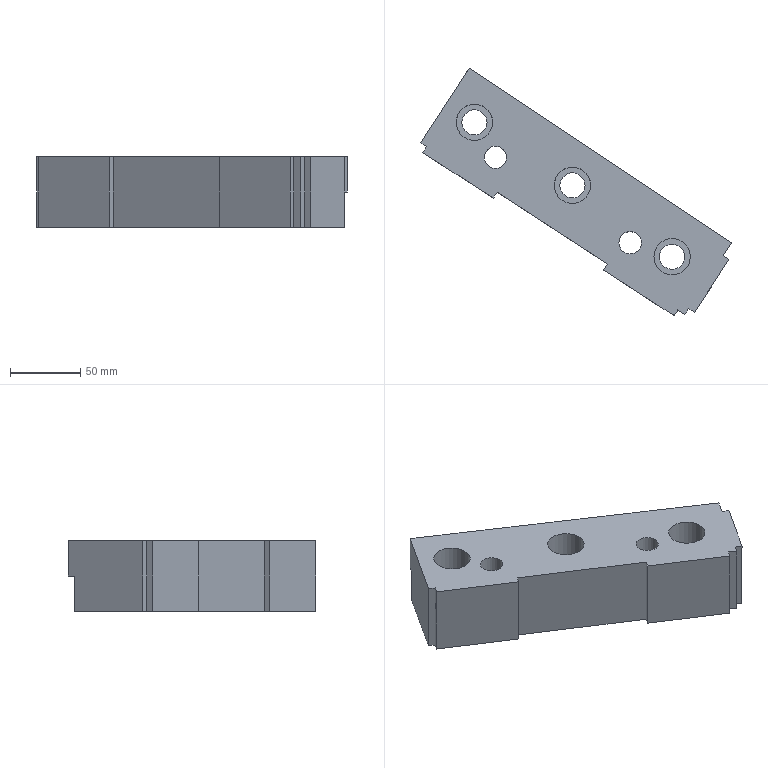Part | NX | features solid 2 | 1 solid | 31 faces | box 221.806 x 176.719 x 50 mm | volume 629014 mm3 | plane 22 | cylinder 8 | spline 1 | commonest cylinder face diameters 18 x3 26 x3 16 x2
STEP:
#1=CARTESIAN_POINT('',(359.804,560.007,-50.));
#2=VERTEX_POINT('',#1);
#3=CARTESIAN_POINT('',(350.804,560.007,-50.));
#4=DIRECTION('',(0.,0.,1.));
#5=DIRECTION('',(1.,0.,0.));
#6=AXIS2_PLACEMENT_3D('',#3,#4,#5);
#7=CIRCLE('',#6,9.);
#8=EDGE_CURVE('',#2,#2,#7,.T.);
#9=ORIENTED_EDGE('',*,*,#8,.F.);
#10=EDGE_LOOP('',(#9));
#11=FACE_BOUND('',#10,.T.);
#12=CARTESIAN_POINT('',(359.804,560.007,-30.));
#13=VERTEX_POINT('',#12);
#14=CARTESIAN_POINT('',(350.804,560.007,-30.));
#15=DIRECTION('',(0.,0.,1.));
#16=DIRECTION('',(1.,0.,0.));
#17=AXIS2_PLACEMENT_3D('',#14,#15,#16);
#18=CIRCLE('',#17,9.);
#19=EDGE_CURVE('',#13,#13,#18,.F.);
#20=ORIENTED_EDGE('',*,*,#19,.F.);
#21=EDGE_LOOP('',(#20));
#22=FACE_BOUND('',#21,.T.);
#23=CARTESIAN_POINT('',(350.804,560.007,-125.));
#24=DIRECTION('',(0.,0.,1.));
#25=DIRECTION('',(1.,0.,0.));
#26=AXIS2_PLACEMENT_3D('',#23,#24,#25);
#27=CYLINDRICAL_SURFACE('',#26,9.);
#28=ADVANCED_FACE('',(#11,#22),#27,.F.);
#29=CARTESIAN_POINT('',(429.804,515.007,-50.));
#30=VERTEX_POINT('',#29);
#31=CARTESIAN_POINT('',(420.804,515.007,-50.));
#32=DIRECTION('',(0.,0.,1.));
#33=DIRECTION('',(1.,0.,0.));
#34=AXIS2_PLACEMENT_3D('',#31,#32,#33);
#35=CIRCLE('',#34,9.);
#36=EDGE_CURVE('',#30,#30,#35,.T.);
#37=ORIENTED_EDGE('',*,*,#36,.F.);
#38=EDGE_LOOP('',(#37));
#39=FACE_BOUND('',#38,.T.);
#40=CARTESIAN_POINT('',(429.804,515.007,-30.));
#41=VERTEX_POINT('',#40);
#42=CARTESIAN_POINT('',(420.804,515.007,-30.));
#43=DIRECTION('',(0.,0.,1.));
#44=DIRECTION('',(1.,0.,0.));
#45=AXIS2_PLACEMENT_3D('',#42,#43,#44);
#46=CIRCLE('',#45,9.);
#47=EDGE_CURVE('',#41,#41,#46,.F.);
#48=ORIENTED_EDGE('',*,*,#47,.F.);
#49=EDGE_LOOP('',(#48));
#50=FACE_BOUND('',#49,.T.);
#51=CARTESIAN_POINT('',(420.804,515.007,-125.));
#52=DIRECTION('',(0.,0.,1.));
#53=DIRECTION('',(1.,0.,0.));
#54=AXIS2_PLACEMENT_3D('',#51,#52,#53);
#55=CYLINDRICAL_SURFACE('',#54,9.);
#56=ADVANCED_FACE('',(#39,#50),#55,.F.);
#57=CARTESIAN_POINT('',(501.017,464.018,-50.));
#58=VERTEX_POINT('',#57);
#59=CARTESIAN_POINT('',(492.017,464.018,-50.));
#60=DIRECTION('',(0.,0.,1.));
#61=DIRECTION('',(1.,0.,0.));
#62=AXIS2_PLACEMENT_3D('',#59,#60,#61);
#63=CIRCLE('',#62,9.);
#64=EDGE_CURVE('',#58,#58,#63,.T.);
#65=ORIENTED_EDGE('',*,*,#64,.F.);
#66=EDGE_LOOP('',(#65));
#67=FACE_BOUND('',#66,.T.);
#68=CARTESIAN_POINT('',(501.017,464.018,-30.));
#69=VERTEX_POINT('',#68);
#70=CARTESIAN_POINT('',(492.017,464.018,-30.));
#71=DIRECTION('',(0.,0.,1.));
#72=DIRECTION('',(1.,0.,0.));
#73=AXIS2_PLACEMENT_3D('',#70,#71,#72);
#74=CIRCLE('',#73,9.);
#75=EDGE_CURVE('',#69,#69,#74,.F.);
#76=ORIENTED_EDGE('',*,*,#75,.F.);
#77=EDGE_LOOP('',(#76));
#78=FACE_BOUND('',#77,.T.);
#79=CARTESIAN_POINT('',(492.017,464.018,-125.));
#80=DIRECTION('',(0.,0.,1.));
#81=DIRECTION('',(1.,0.,0.));
#82=AXIS2_PLACEMENT_3D('',#79,#80,#81);
#83=CYLINDRICAL_SURFACE('',#82,9.);
#84=ADVANCED_FACE('',(#67,#78),#83,.F.);
#85=CARTESIAN_POINT('',(503.876,427.045,-50.));
#86=VERTEX_POINT('',#85);
#87=CARTESIAN_POINT('',(503.876,427.045,0.));
#88=VERTEX_POINT('',#87);
#89=CARTESIAN_POINT('',(503.876,427.045,-50.));
#90=DIRECTION('',(0.,0.,1.));
#91=VECTOR('',#90,1000.);
#92=LINE('',#89,#91);
#93=EDGE_CURVE('',#86,#88,#92,.T.);
#94=ORIENTED_EDGE('',*,*,#93,.T.);
#95=CARTESIAN_POINT('',(501.152,422.852,0.));
#96=VERTEX_POINT('',#95);
#97=CARTESIAN_POINT('',(513.949,442.557,0.));
#98=DIRECTION('',(0.5446,0.8387,0.));
#99=VECTOR('',#98,1000.);
#100=LINE('',#97,#99);
#101=EDGE_CURVE('',#96,#88,#100,.T.);
#102=ORIENTED_EDGE('',*,*,#101,.F.);
#103=CARTESIAN_POINT('',(501.152,422.852,-50.));
#104=VERTEX_POINT('',#103);
#105=CARTESIAN_POINT('',(501.152,422.852,-70.));
#106=DIRECTION('',(0.,0.,1.));
#107=VECTOR('',#106,1000.);
#108=LINE('',#105,#107);
#109=EDGE_CURVE('',#104,#96,#108,.T.);
#110=ORIENTED_EDGE('',*,*,#109,.F.);
#111=CARTESIAN_POINT('',(874.688,998.046,-50.));
#112=DIRECTION('',(-0.5446,-0.8387,0.));
#113=VECTOR('',#112,1000.);
#114=LINE('',#111,#113);
#115=EDGE_CURVE('',#86,#104,#114,.T.);
#116=ORIENTED_EDGE('',*,*,#115,.F.);
#117=EDGE_LOOP('',(#94,#102,#110,#116));
#118=FACE_BOUND('',#117,.T.);
#119=CARTESIAN_POINT('',(1248.625,1573.86,-70.));
#120=DIRECTION('',(-0.8387,0.5446,0.));
#121=DIRECTION('',(-0.5446,-0.8387,0.));
#122=AXIS2_PLACEMENT_3D('',#119,#120,#121);
#123=PLANE('',#122);
#124=ADVANCED_FACE('',(#118),#123,.F.);
#125=CARTESIAN_POINT('',(366.965,509.994,-50.));
#126=VERTEX_POINT('',#125);
#127=CARTESIAN_POINT('',(445.8,458.798,-50.));
#128=VERTEX_POINT('',#127);
#129=CARTESIAN_POINT('',(-52.93,782.677,-50.));
#130=DIRECTION('',(0.8387,-0.5446,0.));
#131=VECTOR('',#130,1000.);
#132=LINE('',#129,#131);
#133=EDGE_CURVE('',#126,#128,#132,.T.);
#134=ORIENTED_EDGE('',*,*,#133,.T.);
#135=CARTESIAN_POINT('',(445.8,458.798,0.));
#136=VERTEX_POINT('',#135);
#137=CARTESIAN_POINT('',(445.8,458.798,-70.));
#138=DIRECTION('',(0.,0.,1.));
#139=VECTOR('',#138,1000.);
#140=LINE('',#137,#139);
#141=EDGE_CURVE('',#128,#136,#140,.T.);
#142=ORIENTED_EDGE('',*,*,#141,.T.);
#143=CARTESIAN_POINT('',(366.965,509.994,0.));
#144=VERTEX_POINT('',#143);
#145=CARTESIAN_POINT('',(-52.93,782.677,0.));
#146=DIRECTION('',(0.8387,-0.5446,0.));
#147=VECTOR('',#146,1000.);
#148=LINE('',#145,#147);
#149=EDGE_CURVE('',#144,#136,#148,.T.);
#150=ORIENTED_EDGE('',*,*,#149,.F.);
#151=CARTESIAN_POINT('',(366.965,509.994,-70.));
#152=DIRECTION('',(0.,0.,1.));
#153=VECTOR('',#152,1000.);
#154=LINE('',#151,#153);
#155=EDGE_CURVE('',#126,#144,#154,.T.);
#156=ORIENTED_EDGE('',*,*,#155,.F.);
#157=EDGE_LOOP('',(#134,#142,#150,#156));
#158=FACE_BOUND('',#157,.T.);
#159=CARTESIAN_POINT('',(-1335.727,1615.736,-70.));
#160=DIRECTION('',(-0.5446,-0.8387,0.));
#161=DIRECTION('',(0.8387,-0.5446,0.));
#162=AXIS2_PLACEMENT_3D('',#159,#160,#161);
#163=PLANE('',#162);
#164=ADVANCED_FACE('',(#158),#163,.T.);
#165=CARTESIAN_POINT('',(312.451,545.396,-50.));
#166=VERTEX_POINT('',#165);
#167=CARTESIAN_POINT('',(316.645,542.673,-50.));
#168=VERTEX_POINT('',#167);
#169=CARTESIAN_POINT('',(-52.93,782.677,-50.));
#170=DIRECTION('',(0.8387,-0.5446,0.));
#171=VECTOR('',#170,1000.);
#172=LINE('',#169,#171);
#173=EDGE_CURVE('',#166,#168,#172,.T.);
#174=ORIENTED_EDGE('',*,*,#173,.T.);
#175=CARTESIAN_POINT('',(316.645,542.673,0.));
#176=VERTEX_POINT('',#175);
#177=CARTESIAN_POINT('',(316.645,542.673,-70.));
#178=DIRECTION('',(0.,0.,1.));
#179=VECTOR('',#178,1000.);
#180=LINE('',#177,#179);
#181=EDGE_CURVE('',#168,#176,#180,.T.);
#182=ORIENTED_EDGE('',*,*,#181,.T.);
#183=CARTESIAN_POINT('',(312.451,545.396,0.));
#184=VERTEX_POINT('',#183);
#185=CARTESIAN_POINT('',(-52.93,782.677,0.));
#186=DIRECTION('',(0.8387,-0.5446,0.));
#187=VECTOR('',#186,1000.);
#188=LINE('',#185,#187);
#189=EDGE_CURVE('',#184,#176,#188,.T.);
#190=ORIENTED_EDGE('',*,*,#189,.F.);
#191=CARTESIAN_POINT('',(312.451,545.396,-70.));
#192=DIRECTION('',(0.,0.,1.));
#193=VECTOR('',#192,1000.);
#194=LINE('',#191,#193);
#195=EDGE_CURVE('',#166,#184,#194,.T.);
#196=ORIENTED_EDGE('',*,*,#195,.F.);
#197=EDGE_LOOP('',(#174,#182,#190,#196));
#198=FACE_BOUND('',#197,.T.);
#199=CARTESIAN_POINT('',(-1335.727,1615.736,-70.));
#200=DIRECTION('',(-0.5446,-0.8387,0.));
#201=DIRECTION('',(0.8387,-0.5446,0.));
#202=AXIS2_PLACEMENT_3D('',#199,#200,#201);
#203=PLANE('',#202);
#204=ADVANCED_FACE('',(#198),#203,.T.);
#205=CARTESIAN_POINT('',(496.12,426.12,-50.));
#206=VERTEX_POINT('',#205);
#207=CARTESIAN_POINT('',(496.12,426.12,0.));
#208=VERTEX_POINT('',#207);
#209=CARTESIAN_POINT('',(496.12,426.12,-70.));
#210=DIRECTION('',(0.,0.,1.));
#211=VECTOR('',#210,1000.);
#212=LINE('',#209,#211);
#213=EDGE_CURVE('',#206,#208,#212,.T.);
#214=ORIENTED_EDGE('',*,*,#213,.F.);
#215=CARTESIAN_POINT('',(-52.93,782.677,-50.));
#216=DIRECTION('',(0.8387,-0.5446,0.));
#217=VECTOR('',#216,1000.);
#218=LINE('',#215,#217);
#219=EDGE_CURVE('',#206,#104,#218,.T.);
#220=ORIENTED_EDGE('',*,*,#219,.T.);
#221=ORIENTED_EDGE('',*,*,#109,.T.);
#222=CARTESIAN_POINT('',(-52.93,782.677,0.));
#223=DIRECTION('',(0.8387,-0.5446,0.));
#224=VECTOR('',#223,1000.);
#225=LINE('',#222,#224);
#226=EDGE_CURVE('',#208,#96,#225,.T.);
#227=ORIENTED_EDGE('',*,*,#226,.F.);
#228=EDGE_LOOP('',(#214,#220,#221,#227));
#229=FACE_BOUND('',#228,.T.);
#230=CARTESIAN_POINT('',(-1335.727,1615.736,-70.));
#231=DIRECTION('',(-0.5446,-0.8387,0.));
#232=DIRECTION('',(0.8387,-0.5446,0.));
#233=AXIS2_PLACEMENT_3D('',#230,#231,#232);
#234=PLANE('',#233);
#235=ADVANCED_FACE('',(#229),#234,.T.);
#236=ORIENTED_EDGE('',*,*,#195,.T.);
#237=CARTESIAN_POINT('',(347.032,598.645,0.));
#238=VERTEX_POINT('',#237);
#239=CARTESIAN_POINT('',(685.987,1120.59,0.));
#240=DIRECTION('',(-0.5446,-0.8387,0.));
#241=VECTOR('',#240,1000.);
#242=LINE('',#239,#241);
#243=EDGE_CURVE('',#238,#184,#242,.T.);
#244=ORIENTED_EDGE('',*,*,#243,.F.);
#245=CARTESIAN_POINT('',(347.032,598.645,-25.));
#246=VERTEX_POINT('',#245);
#247=CARTESIAN_POINT('',(347.032,598.645,-70.));
#248=DIRECTION('',(0.,0.,1.));
#249=VECTOR('',#248,1000.);
#250=LINE('',#247,#249);
#251=EDGE_CURVE('',#246,#238,#250,.T.);
#252=ORIENTED_EDGE('',*,*,#251,.F.);
#253=CARTESIAN_POINT('',(344.309,594.452,-25.));
#254=VERTEX_POINT('',#253);
#255=CARTESIAN_POINT('',(1059.925,1696.404,-25.));
#256=DIRECTION('',(-0.5446,-0.8387,0.));
#257=VECTOR('',#256,1000.);
#258=LINE('',#255,#257);
#259=EDGE_CURVE('',#246,#254,#258,.T.);
#260=ORIENTED_EDGE('',*,*,#259,.T.);
#261=CARTESIAN_POINT('',(344.309,594.452,-50.));
#262=VERTEX_POINT('',#261);
#263=CARTESIAN_POINT('',(344.309,594.452,-70.));
#264=DIRECTION('',(0.,0.,-1.));
#265=VECTOR('',#264,1000.);
#266=LINE('',#263,#265);
#267=EDGE_CURVE('',#254,#262,#266,.T.);
#268=ORIENTED_EDGE('',*,*,#267,.T.);
#269=CARTESIAN_POINT('',(685.987,1120.59,-50.));
#270=DIRECTION('',(-0.5446,-0.8387,0.));
#271=VECTOR('',#270,1000.);
#272=LINE('',#269,#271);
#273=EDGE_CURVE('',#262,#166,#272,.T.);
#274=ORIENTED_EDGE('',*,*,#273,.T.);
#275=EDGE_LOOP('',(#236,#244,#252,#260,#268,#274));
#276=FACE_BOUND('',#275,.T.);
#277=CARTESIAN_POINT('',(1059.925,1696.404,-70.));
#278=DIRECTION('',(-0.8387,0.5446,0.));
#279=DIRECTION('',(-0.5446,-0.8387,0.));
#280=AXIS2_PLACEMENT_3D('',#277,#278,#279);
#281=PLANE('',#280);
#282=ADVANCED_FACE('',(#276),#281,.T.);
#283=CARTESIAN_POINT('',(534.257,473.829,-25.));
#284=VERTEX_POINT('',#283);
#285=CARTESIAN_POINT('',(347.032,598.645,-25.));
#286=DIRECTION('',(0.8321,-0.5547,0.));
#287=VECTOR('',#286,1000.);
#288=LINE('',#285,#287);
#289=EDGE_CURVE('',#246,#284,#288,.T.);
#290=ORIENTED_EDGE('',*,*,#289,.F.);
#291=ORIENTED_EDGE('',*,*,#251,.T.);
#292=CARTESIAN_POINT('',(534.257,473.829,0.));
#293=VERTEX_POINT('',#292);
#294=CARTESIAN_POINT('',(-21.675,844.45,0.));
#295=DIRECTION('',(0.8321,-0.5547,0.));
#296=VECTOR('',#295,1000.);
#297=LINE('',#294,#296);
#298=EDGE_CURVE('',#238,#293,#297,.T.);
#299=ORIENTED_EDGE('',*,*,#298,.T.);
#300=CARTESIAN_POINT('',(534.257,473.829,-70.));
#301=DIRECTION('',(0.,0.,1.));
#302=VECTOR('',#301,1000.);
#303=LINE('',#300,#302);
#304=EDGE_CURVE('',#284,#293,#303,.T.);
#305=ORIENTED_EDGE('',*,*,#304,.F.);
#306=EDGE_LOOP('',(#290,#291,#299,#305));
#307=FACE_BOUND('',#306,.T.);
#308=CARTESIAN_POINT('',(347.032,598.645,-70.));
#309=DIRECTION('',(-0.5547,-0.8321,0.));
#310=DIRECTION('',(0.8321,-0.5547,0.));
#311=AXIS2_PLACEMENT_3D('',#308,#309,#310);
#312=PLANE('',#311);
#313=ADVANCED_FACE('',(#307),#312,.F.);
#314=ORIENTED_EDGE('',*,*,#8,.T.);
#315=EDGE_LOOP('',(#314));
#316=FACE_BOUND('',#315,.T.);
#317=CARTESIAN_POINT('',(373.804,535.007,-50.));
#318=VERTEX_POINT('',#317);
#319=CARTESIAN_POINT('',(365.804,535.007,-50.));
#320=DIRECTION('',(0.,0.,1.));
#321=DIRECTION('',(1.,0.,0.));
#322=AXIS2_PLACEMENT_3D('',#319,#320,#321);
#323=CIRCLE('',#322,8.);
#324=EDGE_CURVE('',#318,#318,#323,.T.);
#325=ORIENTED_EDGE('',*,*,#324,.T.);
#326=EDGE_LOOP('',(#325));
#327=FACE_BOUND('',#326,.T.);
#328=ORIENTED_EDGE('',*,*,#36,.T.);
#329=EDGE_LOOP('',(#328));
#330=FACE_BOUND('',#329,.T.);
#331=CARTESIAN_POINT('',(470.017,474.018,-50.));
#332=VERTEX_POINT('',#331);
#333=CARTESIAN_POINT('',(462.017,474.018,-50.));
#334=DIRECTION('',(0.,0.,1.));
#335=DIRECTION('',(1.,0.,0.));
#336=AXIS2_PLACEMENT_3D('',#333,#334,#335);
#337=CIRCLE('',#336,8.);
#338=EDGE_CURVE('',#332,#332,#337,.T.);
#339=ORIENTED_EDGE('',*,*,#338,.T.);
#340=EDGE_LOOP('',(#339));
#341=FACE_BOUND('',#340,.T.);
#342=ORIENTED_EDGE('',*,*,#64,.T.);
#343=EDGE_LOOP('',(#342));
#344=FACE_BOUND('',#343,.T.);
#345=CARTESIAN_POINT('',(531.534,469.635,-50.));
#346=VERTEX_POINT('',#345);
#347=CARTESIAN_POINT('',(344.309,594.452,-50.));
#348=CARTESIAN_POINT('',(406.717,552.846,-50.));
#349=CARTESIAN_POINT('',(469.125,511.241,-50.));
#350=CARTESIAN_POINT('',(531.534,469.635,-50.));
#351=B_SPLINE_CURVE_WITH_KNOTS('',3,(#347,#348,#349,#350),.UNSPECIFIED.,.F.,.F.,(4,4),(0.,1.),.UNSPECIFIED.);
#352=EDGE_CURVE('',#262,#346,#351,.T.);
#353=ORIENTED_EDGE('',*,*,#352,.T.);
#354=CARTESIAN_POINT('',(528.384,464.786,-50.));
#355=VERTEX_POINT('',#354);
#356=CARTESIAN_POINT('',(874.688,998.046,-50.));
#357=DIRECTION('',(-0.5446,-0.8387,0.));
#358=VECTOR('',#357,1000.);
#359=LINE('',#356,#358);
#360=EDGE_CURVE('',#346,#355,#359,.T.);
#361=ORIENTED_EDGE('',*,*,#360,.T.);
#362=CARTESIAN_POINT('',(532.578,462.062,-50.));
#363=VERTEX_POINT('',#362);
#364=CARTESIAN_POINT('',(528.384,464.786,-50.));
#365=DIRECTION('',(0.8387,-0.5446,0.));
#366=VECTOR('',#365,1000.);
#367=LINE('',#364,#366);
#368=EDGE_CURVE('',#355,#363,#367,.T.);
#369=ORIENTED_EDGE('',*,*,#368,.T.);
#370=CARTESIAN_POINT('',(508.069,424.322,-50.));
#371=VERTEX_POINT('',#370);
#372=CARTESIAN_POINT('',(503.712,417.613,-50.));
#373=DIRECTION('',(0.5446,0.8387,0.));
#374=VECTOR('',#373,1000.);
#375=LINE('',#372,#374);
#376=EDGE_CURVE('',#371,#363,#375,.T.);
#377=ORIENTED_EDGE('',*,*,#376,.F.);
#378=CARTESIAN_POINT('',(503.876,427.045,-50.));
#379=DIRECTION('',(0.8387,-0.5446,0.));
#380=VECTOR('',#379,1000.);
#381=LINE('',#378,#380);
#382=EDGE_CURVE('',#86,#371,#381,.T.);
#383=ORIENTED_EDGE('',*,*,#382,.F.);
#384=ORIENTED_EDGE('',*,*,#115,.T.);
#385=ORIENTED_EDGE('',*,*,#219,.F.);
#386=CARTESIAN_POINT('',(493.397,421.926,-50.));
#387=VERTEX_POINT('',#386);
#388=CARTESIAN_POINT('',(485.228,409.346,-50.));
#389=DIRECTION('',(-0.5446,-0.8387,0.));
#390=VECTOR('',#389,1000.);
#391=LINE('',#388,#390);
#392=EDGE_CURVE('',#206,#387,#391,.T.);
#393=ORIENTED_EDGE('',*,*,#392,.T.);
#394=CARTESIAN_POINT('',(443.077,454.605,-50.));
#395=VERTEX_POINT('',#394);
#396=CARTESIAN_POINT('',(468.237,438.266,-50.));
#397=DIRECTION('',(0.8387,-0.5446,0.));
#398=VECTOR('',#397,1000.);
#399=LINE('',#396,#398);
#400=EDGE_CURVE('',#395,#387,#399,.T.);
#401=ORIENTED_EDGE('',*,*,#400,.F.);
#402=CARTESIAN_POINT('',(434.907,442.025,-50.));
#403=DIRECTION('',(-0.5446,-0.8387,0.));
#404=VECTOR('',#403,1000.);
#405=LINE('',#402,#404);
#406=EDGE_CURVE('',#128,#395,#405,.T.);
#407=ORIENTED_EDGE('',*,*,#406,.F.);
#408=ORIENTED_EDGE('',*,*,#133,.F.);
#409=CARTESIAN_POINT('',(364.242,505.801,-50.));
#410=VERTEX_POINT('',#409);
#411=CARTESIAN_POINT('',(356.072,493.221,-50.));
#412=DIRECTION('',(-0.5446,-0.8387,0.));
#413=VECTOR('',#412,1000.);
#414=LINE('',#411,#413);
#415=EDGE_CURVE('',#126,#410,#414,.T.);
#416=ORIENTED_EDGE('',*,*,#415,.T.);
#417=CARTESIAN_POINT('',(313.922,538.479,-50.));
#418=VERTEX_POINT('',#417);
#419=CARTESIAN_POINT('',(322.308,533.033,-50.));
#420=DIRECTION('',(0.8387,-0.5446,0.));
#421=VECTOR('',#420,1000.);
#422=LINE('',#419,#421);
#423=EDGE_CURVE('',#418,#410,#422,.T.);
#424=ORIENTED_EDGE('',*,*,#423,.F.);
#425=CARTESIAN_POINT('',(305.752,525.899,-50.));
#426=DIRECTION('',(-0.5446,-0.8387,0.));
#427=VECTOR('',#426,1000.);
#428=LINE('',#425,#427);
#429=EDGE_CURVE('',#168,#418,#428,.T.);
#430=ORIENTED_EDGE('',*,*,#429,.F.);
#431=ORIENTED_EDGE('',*,*,#173,.F.);
#432=ORIENTED_EDGE('',*,*,#273,.F.);
#433=EDGE_LOOP('',(#353,#361,#369,#377,#383,#384,#385,#393,#401,#407,#408,#416,#424,#430,#431,#432));
#434=FACE_BOUND('',#433,.T.);
#435=CARTESIAN_POINT('',(320.605,1357.871,-50.));
#436=DIRECTION('',(0.,0.,1.));
#437=DIRECTION('',(1.,0.,0.));
#438=AXIS2_PLACEMENT_3D('',#435,#436,#437);
#439=PLANE('',#438);
#440=ADVANCED_FACE('',(#316,#327,#330,#341,#344,#434),#439,.F.);
#441=CARTESIAN_POINT('',(528.384,464.786,0.));
#442=VERTEX_POINT('',#441);
#443=CARTESIAN_POINT('',(874.688,998.046,0.));
#444=DIRECTION('',(-0.5446,-0.8387,0.));
#445=VECTOR('',#444,1000.);
#446=LINE('',#443,#445);
#447=EDGE_CURVE('',#293,#442,#446,.T.);
#448=ORIENTED_EDGE('',*,*,#447,.T.);
#449=CARTESIAN_POINT('',(528.384,464.786,-50.));
#450=DIRECTION('',(0.,0.,1.));
#451=VECTOR('',#450,1000.);
#452=LINE('',#449,#451);
#453=EDGE_CURVE('',#355,#442,#452,.T.);
#454=ORIENTED_EDGE('',*,*,#453,.F.);
#455=ORIENTED_EDGE('',*,*,#360,.F.);
#456=CARTESIAN_POINT('',(531.534,469.635,-25.));
#457=VERTEX_POINT('',#456);
#458=CARTESIAN_POINT('',(531.534,469.635,-37.5));
#459=DIRECTION('',(0.,0.,-1.));
#460=VECTOR('',#459,1000.);
#461=LINE('',#458,#460);
#462=EDGE_CURVE('',#457,#346,#461,.T.);
#463=ORIENTED_EDGE('',*,*,#462,.F.);
#464=CARTESIAN_POINT('',(1248.625,1573.86,-25.));
#465=DIRECTION('',(-0.5446,-0.8387,0.));
#466=VECTOR('',#465,1000.);
#467=LINE('',#464,#466);
#468=EDGE_CURVE('',#284,#457,#467,.T.);
#469=ORIENTED_EDGE('',*,*,#468,.F.);
#470=ORIENTED_EDGE('',*,*,#304,.T.);
#471=EDGE_LOOP('',(#448,#454,#455,#463,#469,#470));
#472=FACE_BOUND('',#471,.T.);
#473=CARTESIAN_POINT('',(1248.625,1573.86,-70.));
#474=DIRECTION('',(-0.8387,0.5446,0.));
#475=DIRECTION('',(-0.5446,-0.8387,0.));
#476=AXIS2_PLACEMENT_3D('',#473,#474,#475);
#477=PLANE('',#476);
#478=ADVANCED_FACE('',(#472),#477,.F.);
#479=ORIENTED_EDGE('',*,*,#243,.T.);
#480=ORIENTED_EDGE('',*,*,#189,.T.);
#481=CARTESIAN_POINT('',(313.922,538.479,0.));
#482=VERTEX_POINT('',#481);
#483=CARTESIAN_POINT('',(329.441,562.378,0.));
#484=DIRECTION('',(-0.5446,-0.8387,0.));
#485=VECTOR('',#484,1000.);
#486=LINE('',#483,#485);
#487=EDGE_CURVE('',#176,#482,#486,.T.);
#488=ORIENTED_EDGE('',*,*,#487,.T.);
#489=CARTESIAN_POINT('',(364.242,505.801,0.));
#490=VERTEX_POINT('',#489);
#491=CARTESIAN_POINT('',(322.308,533.033,0.));
#492=DIRECTION('',(0.8387,-0.5446,0.));
#493=VECTOR('',#492,1000.);
#494=LINE('',#491,#493);
#495=EDGE_CURVE('',#482,#490,#494,.T.);
#496=ORIENTED_EDGE('',*,*,#495,.T.);
#497=CARTESIAN_POINT('',(379.762,529.699,0.));
#498=DIRECTION('',(-0.5446,-0.8387,0.));
#499=VECTOR('',#498,1000.);
#500=LINE('',#497,#499);
#501=EDGE_CURVE('',#144,#490,#500,.T.);
#502=ORIENTED_EDGE('',*,*,#501,.F.);
#503=ORIENTED_EDGE('',*,*,#149,.T.);
#504=CARTESIAN_POINT('',(443.077,454.605,0.));
#505=VERTEX_POINT('',#504);
#506=CARTESIAN_POINT('',(458.597,478.503,0.));
#507=DIRECTION('',(-0.5446,-0.8387,0.));
#508=VECTOR('',#507,1000.);
#509=LINE('',#506,#508);
#510=EDGE_CURVE('',#136,#505,#509,.T.);
#511=ORIENTED_EDGE('',*,*,#510,.T.);
#512=CARTESIAN_POINT('',(493.397,421.926,0.));
#513=VERTEX_POINT('',#512);
#514=CARTESIAN_POINT('',(468.237,438.266,0.));
#515=DIRECTION('',(0.8387,-0.5446,0.));
#516=VECTOR('',#515,1000.);
#517=LINE('',#514,#516);
#518=EDGE_CURVE('',#505,#513,#517,.T.);
#519=ORIENTED_EDGE('',*,*,#518,.T.);
#520=CARTESIAN_POINT('',(508.917,445.825,0.));
#521=DIRECTION('',(-0.5446,-0.8387,0.));
#522=VECTOR('',#521,1000.);
#523=LINE('',#520,#522);
#524=EDGE_CURVE('',#208,#513,#523,.T.);
#525=ORIENTED_EDGE('',*,*,#524,.F.);
#526=ORIENTED_EDGE('',*,*,#226,.T.);
#527=ORIENTED_EDGE('',*,*,#101,.T.);
#528=CARTESIAN_POINT('',(508.069,424.322,0.));
#529=VERTEX_POINT('',#528);
#530=CARTESIAN_POINT('',(503.876,427.045,0.));
#531=DIRECTION('',(0.8387,-0.5446,0.));
#532=VECTOR('',#531,1000.);
#533=LINE('',#530,#532);
#534=EDGE_CURVE('',#88,#529,#533,.T.);
#535=ORIENTED_EDGE('',*,*,#534,.T.);
#536=CARTESIAN_POINT('',(532.578,462.062,0.));
#537=VERTEX_POINT('',#536);
#538=CARTESIAN_POINT('',(518.142,439.834,0.));
#539=DIRECTION('',(0.5446,0.8387,0.));
#540=VECTOR('',#539,1000.);
#541=LINE('',#538,#540);
#542=EDGE_CURVE('',#529,#537,#541,.T.);
#543=ORIENTED_EDGE('',*,*,#542,.T.);
#544=CARTESIAN_POINT('',(528.384,464.786,0.));
#545=DIRECTION('',(0.8387,-0.5446,0.));
#546=VECTOR('',#545,1000.);
#547=LINE('',#544,#546);
#548=EDGE_CURVE('',#442,#537,#547,.T.);
#549=ORIENTED_EDGE('',*,*,#548,.F.);
#550=ORIENTED_EDGE('',*,*,#447,.F.);
#551=ORIENTED_EDGE('',*,*,#298,.F.);
#552=EDGE_LOOP('',(#479,#480,#488,#496,#502,#503,#511,#519,#525,#526,#527,#535,#543,#549,#550,#551));
#553=FACE_BOUND('',#552,.T.);
#554=CARTESIAN_POINT('',(337.804,560.007,0.));
#555=VERTEX_POINT('',#554);
#556=CARTESIAN_POINT('',(350.804,560.007,0.));
#557=DIRECTION('',(0.,0.,-1.));
#558=DIRECTION('',(-1.,0.,0.));
#559=AXIS2_PLACEMENT_3D('',#556,#557,#558);
#560=CIRCLE('',#559,13.);
#561=EDGE_CURVE('',#555,#555,#560,.F.);
#562=ORIENTED_EDGE('',*,*,#561,.F.);
#563=EDGE_LOOP('',(#562));
#564=FACE_BOUND('',#563,.T.);
#565=CARTESIAN_POINT('',(407.804,515.007,0.));
#566=VERTEX_POINT('',#565);
#567=CARTESIAN_POINT('',(420.804,515.007,0.));
#568=DIRECTION('',(0.,0.,-1.));
#569=DIRECTION('',(-1.,0.,0.));
#570=AXIS2_PLACEMENT_3D('',#567,#568,#569);
#571=CIRCLE('',#570,13.);
#572=EDGE_CURVE('',#566,#566,#571,.F.);
#573=ORIENTED_EDGE('',*,*,#572,.F.);
#574=EDGE_LOOP('',(#573));
#575=FACE_BOUND('',#574,.T.);
#576=CARTESIAN_POINT('',(479.017,464.018,0.));
#577=VERTEX_POINT('',#576);
#578=CARTESIAN_POINT('',(492.017,464.018,0.));
#579=DIRECTION('',(0.,0.,-1.));
#580=DIRECTION('',(-1.,0.,0.));
#581=AXIS2_PLACEMENT_3D('',#578,#579,#580);
#582=CIRCLE('',#581,13.);
#583=EDGE_CURVE('',#577,#577,#582,.F.);
#584=ORIENTED_EDGE('',*,*,#583,.F.);
#585=EDGE_LOOP('',(#584));
#586=FACE_BOUND('',#585,.T.);
#587=CARTESIAN_POINT('',(357.804,535.007,0.));
#588=VERTEX_POINT('',#587);
#589=CARTESIAN_POINT('',(365.804,535.007,0.));
#590=DIRECTION('',(0.,0.,-1.));
#591=DIRECTION('',(-1.,0.,0.));
#592=AXIS2_PLACEMENT_3D('',#589,#590,#591);
#593=CIRCLE('',#592,8.);
#594=EDGE_CURVE('',#588,#588,#593,.F.);
#595=ORIENTED_EDGE('',*,*,#594,.F.);
#596=EDGE_LOOP('',(#595));
#597=FACE_BOUND('',#596,.T.);
#598=CARTESIAN_POINT('',(454.017,474.018,0.));
#599=VERTEX_POINT('',#598);
#600=CARTESIAN_POINT('',(462.017,474.018,0.));
#601=DIRECTION('',(0.,0.,-1.));
#602=DIRECTION('',(-1.,0.,0.));
#603=AXIS2_PLACEMENT_3D('',#600,#601,#602);
#604=CIRCLE('',#603,8.);
#605=EDGE_CURVE('',#599,#599,#604,.F.);
#606=ORIENTED_EDGE('',*,*,#605,.F.);
#607=EDGE_LOOP('',(#606));
#608=FACE_BOUND('',#607,.T.);
#609=CARTESIAN_POINT('',(320.605,1357.871,0.));
#610=DIRECTION('',(0.,0.,1.));
#611=DIRECTION('',(1.,0.,0.));
#612=AXIS2_PLACEMENT_3D('',#609,#610,#611);
#613=PLANE('',#612);
#614=ADVANCED_FACE('',(#553,#564,#575,#586,#597,#608),#613,.T.);
#615=CARTESIAN_POINT('',(344.309,594.452,-25.));
#616=CARTESIAN_POINT('',(406.717,552.846,-25.));
#617=CARTESIAN_POINT('',(469.125,511.241,-25.));
#618=CARTESIAN_POINT('',(531.534,469.635,-25.));
#619=B_SPLINE_CURVE_WITH_KNOTS('',3,(#615,#616,#617,#618),.UNSPECIFIED.,.F.,.F.,(4,4),(0.9632,1.188),.UNSPECIFIED.);
#620=EDGE_CURVE('',#254,#457,#619,.T.);
#621=ORIENTED_EDGE('',*,*,#620,.T.);
#622=ORIENTED_EDGE('',*,*,#462,.T.);
#623=ORIENTED_EDGE('',*,*,#352,.F.);
#624=ORIENTED_EDGE('',*,*,#267,.F.);
#625=EDGE_LOOP('',(#621,#622,#623,#624));
#626=FACE_BOUND('',#625,.T.);
#627=CARTESIAN_POINT('',(344.309,594.452,-25.));
#628=CARTESIAN_POINT('',(344.309,594.452,-50.));
#629=CARTESIAN_POINT('',(411.082,549.936,-25.));
#630=CARTESIAN_POINT('',(411.082,549.936,-50.));
#631=CARTESIAN_POINT('',(465.216,513.847,-25.));
#632=CARTESIAN_POINT('',(465.216,513.847,-50.));
#633=CARTESIAN_POINT('',(531.534,469.635,-25.));
#634=CARTESIAN_POINT('',(531.534,469.635,-50.));
#635=B_SPLINE_SURFACE_WITH_KNOTS('',3,1,((#627,#628),(#629,#630),(#631,#632),(#633,#634)),.SURF_OF_LINEAR_EXTRUSION.,.F.,.F.,.F.,(4,4),(2,2),(0.0002501,1.),(0.,1.),.PIECEWISE_BEZIER_KNOTS.);
#636=ADVANCED_FACE('',(#626),#635,.T.);
#637=ORIENTED_EDGE('',*,*,#289,.T.);
#638=ORIENTED_EDGE('',*,*,#468,.T.);
#639=ORIENTED_EDGE('',*,*,#620,.F.);
#640=ORIENTED_EDGE('',*,*,#259,.F.);
#641=EDGE_LOOP('',(#637,#638,#639,#640));
#642=FACE_BOUND('',#641,.T.);
#643=CARTESIAN_POINT('',(347.032,598.645,-25.));
#644=DIRECTION('',(0.,0.,-1.));
#645=DIRECTION('',(-1.,0.,0.));
#646=AXIS2_PLACEMENT_3D('',#643,#644,#645);
#647=PLANE('',#646);
#648=ADVANCED_FACE('',(#642),#647,.T.);
#649=CARTESIAN_POINT('',(364.242,505.801,-50.));
#650=DIRECTION('',(0.,0.,1.));
#651=VECTOR('',#650,1000.);
#652=LINE('',#649,#651);
#653=EDGE_CURVE('',#410,#490,#652,.T.);
#654=ORIENTED_EDGE('',*,*,#653,.F.);
#655=ORIENTED_EDGE('',*,*,#415,.F.);
#656=ORIENTED_EDGE('',*,*,#155,.T.);
#657=ORIENTED_EDGE('',*,*,#501,.T.);
#658=EDGE_LOOP('',(#654,#655,#656,#657));
#659=FACE_BOUND('',#658,.T.);
#660=CARTESIAN_POINT('',(356.072,493.221,-50.));
#661=DIRECTION('',(0.8387,-0.5446,0.));
#662=DIRECTION('',(0.5446,0.8387,0.));
#663=AXIS2_PLACEMENT_3D('',#660,#661,#662);
#664=PLANE('',#663);
#665=ADVANCED_FACE('',(#659),#664,.T.);
#666=CARTESIAN_POINT('',(313.922,538.479,-50.));
#667=DIRECTION('',(0.,0.,1.));
#668=VECTOR('',#667,1000.);
#669=LINE('',#666,#668);
#670=EDGE_CURVE('',#418,#482,#669,.T.);
#671=ORIENTED_EDGE('',*,*,#670,.T.);
#672=ORIENTED_EDGE('',*,*,#487,.F.);
#673=ORIENTED_EDGE('',*,*,#181,.F.);
#674=ORIENTED_EDGE('',*,*,#429,.T.);
#675=EDGE_LOOP('',(#671,#672,#673,#674));
#676=FACE_BOUND('',#675,.T.);
#677=CARTESIAN_POINT('',(305.752,525.899,-50.));
#678=DIRECTION('',(0.8387,-0.5446,0.));
#679=DIRECTION('',(0.5446,0.8387,0.));
#680=AXIS2_PLACEMENT_3D('',#677,#678,#679);
#681=PLANE('',#680);
#682=ADVANCED_FACE('',(#676),#681,.F.);
#683=ORIENTED_EDGE('',*,*,#653,.T.);
#684=ORIENTED_EDGE('',*,*,#495,.F.);
#685=ORIENTED_EDGE('',*,*,#670,.F.);
#686=ORIENTED_EDGE('',*,*,#423,.T.);
#687=EDGE_LOOP('',(#683,#684,#685,#686));
#688=FACE_BOUND('',#687,.T.);
#689=CARTESIAN_POINT('',(322.308,533.033,-50.));
#690=DIRECTION('',(0.5446,0.8387,0.));
#691=DIRECTION('',(0.,0.,1.));
#692=AXIS2_PLACEMENT_3D('',#689,#690,#691);
#693=PLANE('',#692);
#694=ADVANCED_FACE('',(#688),#693,.F.);
#695=CARTESIAN_POINT('',(493.397,421.926,-50.));
#696=DIRECTION('',(0.,0.,1.));
#697=VECTOR('',#696,1000.);
#698=LINE('',#695,#697);
#699=EDGE_CURVE('',#387,#513,#698,.T.);
#700=ORIENTED_EDGE('',*,*,#699,.F.);
#701=ORIENTED_EDGE('',*,*,#392,.F.);
#702=ORIENTED_EDGE('',*,*,#213,.T.);
#703=ORIENTED_EDGE('',*,*,#524,.T.);
#704=EDGE_LOOP('',(#700,#701,#702,#703));
#705=FACE_BOUND('',#704,.T.);
#706=CARTESIAN_POINT('',(485.228,409.346,-50.));
#707=DIRECTION('',(0.8387,-0.5446,0.));
#708=DIRECTION('',(0.5446,0.8387,0.));
#709=AXIS2_PLACEMENT_3D('',#706,#707,#708);
#710=PLANE('',#709);
#711=ADVANCED_FACE('',(#705),#710,.T.);
#712=CARTESIAN_POINT('',(443.077,454.605,-50.));
#713=DIRECTION('',(0.,0.,1.));
#714=VECTOR('',#713,1000.);
#715=LINE('',#712,#714);
#716=EDGE_CURVE('',#395,#505,#715,.T.);
#717=ORIENTED_EDGE('',*,*,#716,.T.);
#718=ORIENTED_EDGE('',*,*,#510,.F.);
#719=ORIENTED_EDGE('',*,*,#141,.F.);
#720=ORIENTED_EDGE('',*,*,#406,.T.);
#721=EDGE_LOOP('',(#717,#718,#719,#720));
#722=FACE_BOUND('',#721,.T.);
#723=CARTESIAN_POINT('',(434.907,442.025,-50.));
#724=DIRECTION('',(0.8387,-0.5446,0.));
#725=DIRECTION('',(0.5446,0.8387,0.));
#726=AXIS2_PLACEMENT_3D('',#723,#724,#725);
#727=PLANE('',#726);
#728=ADVANCED_FACE('',(#722),#727,.F.);
#729=ORIENTED_EDGE('',*,*,#699,.T.);
#730=ORIENTED_EDGE('',*,*,#518,.F.);
#731=ORIENTED_EDGE('',*,*,#716,.F.);
#732=ORIENTED_EDGE('',*,*,#400,.T.);
#733=EDGE_LOOP('',(#729,#730,#731,#732));
#734=FACE_BOUND('',#733,.T.);
#735=CARTESIAN_POINT('',(468.237,438.266,-50.));
#736=DIRECTION('',(0.5446,0.8387,0.));
#737=DIRECTION('',(0.,0.,1.));
#738=AXIS2_PLACEMENT_3D('',#735,#736,#737);
#739=PLANE('',#738);
#740=ADVANCED_FACE('',(#734),#739,.F.);
#741=CARTESIAN_POINT('',(532.578,462.062,-50.));
#742=DIRECTION('',(0.,0.,1.));
#743=VECTOR('',#742,1000.);
#744=LINE('',#741,#743);
#745=EDGE_CURVE('',#363,#537,#744,.T.);
#746=ORIENTED_EDGE('',*,*,#745,.F.);
#747=ORIENTED_EDGE('',*,*,#368,.F.);
#748=ORIENTED_EDGE('',*,*,#453,.T.);
#749=ORIENTED_EDGE('',*,*,#548,.T.);
#750=EDGE_LOOP('',(#746,#747,#748,#749));
#751=FACE_BOUND('',#750,.T.);
#752=CARTESIAN_POINT('',(528.384,464.786,-50.));
#753=DIRECTION('',(0.5446,0.8387,0.));
#754=DIRECTION('',(-0.8387,0.5446,0.));
#755=AXIS2_PLACEMENT_3D('',#752,#753,#754);
#756=PLANE('',#755);
#757=ADVANCED_FACE('',(#751),#756,.T.);
#758=CARTESIAN_POINT('',(508.069,424.322,-50.));
#759=DIRECTION('',(0.,0.,1.));
#760=VECTOR('',#759,1000.);
#761=LINE('',#758,#760);
#762=EDGE_CURVE('',#371,#529,#761,.T.);
#763=ORIENTED_EDGE('',*,*,#762,.T.);
#764=ORIENTED_EDGE('',*,*,#534,.F.);
#765=ORIENTED_EDGE('',*,*,#93,.F.);
#766=ORIENTED_EDGE('',*,*,#382,.T.);
#767=EDGE_LOOP('',(#763,#764,#765,#766));
#768=FACE_BOUND('',#767,.T.);
#769=CARTESIAN_POINT('',(503.876,427.045,-50.));
#770=DIRECTION('',(0.5446,0.8387,0.));
#771=DIRECTION('',(-0.8387,0.5446,0.));
#772=AXIS2_PLACEMENT_3D('',#769,#770,#771);
#773=PLANE('',#772);
#774=ADVANCED_FACE('',(#768),#773,.F.);
#775=ORIENTED_EDGE('',*,*,#745,.T.);
#776=ORIENTED_EDGE('',*,*,#542,.F.);
#777=ORIENTED_EDGE('',*,*,#762,.F.);
#778=ORIENTED_EDGE('',*,*,#376,.T.);
#779=EDGE_LOOP('',(#775,#776,#777,#778));
#780=FACE_BOUND('',#779,.T.);
#781=CARTESIAN_POINT('',(503.712,417.613,-50.));
#782=DIRECTION('',(-0.8387,0.5446,0.));
#783=DIRECTION('',(0.,0.,1.));
#784=AXIS2_PLACEMENT_3D('',#781,#782,#783);
#785=PLANE('',#784);
#786=ADVANCED_FACE('',(#780),#785,.F.);
#787=ORIENTED_EDGE('',*,*,#605,.T.);
#788=EDGE_LOOP('',(#787));
#789=FACE_BOUND('',#788,.T.);
#790=ORIENTED_EDGE('',*,*,#338,.F.);
#791=EDGE_LOOP('',(#790));
#792=FACE_BOUND('',#791,.T.);
#793=CARTESIAN_POINT('',(462.017,474.018,-125.));
#794=DIRECTION('',(0.,0.,1.));
#795=DIRECTION('',(1.,0.,0.));
#796=AXIS2_PLACEMENT_3D('',#793,#794,#795);
#797=CYLINDRICAL_SURFACE('',#796,8.);
#798=ADVANCED_FACE('',(#789,#792),#797,.F.);
#799=ORIENTED_EDGE('',*,*,#594,.T.);
#800=EDGE_LOOP('',(#799));
#801=FACE_BOUND('',#800,.T.);
#802=ORIENTED_EDGE('',*,*,#324,.F.);
#803=EDGE_LOOP('',(#802));
#804=FACE_BOUND('',#803,.T.);
#805=CARTESIAN_POINT('',(365.804,535.007,-125.));
#806=DIRECTION('',(0.,0.,1.));
#807=DIRECTION('',(1.,0.,0.));
#808=AXIS2_PLACEMENT_3D('',#805,#806,#807);
#809=CYLINDRICAL_SURFACE('',#808,8.);
#810=ADVANCED_FACE('',(#801,#804),#809,.F.);
#811=CARTESIAN_POINT('',(505.017,464.018,-30.));
#812=VERTEX_POINT('',#811);
#813=CARTESIAN_POINT('',(492.017,464.018,-30.));
#814=DIRECTION('',(0.,0.,1.));
#815=DIRECTION('',(1.,0.,0.));
#816=AXIS2_PLACEMENT_3D('',#813,#814,#815);
#817=CIRCLE('',#816,13.);
#818=EDGE_CURVE('',#812,#812,#817,.T.);
#819=ORIENTED_EDGE('',*,*,#818,.T.);
#820=EDGE_LOOP('',(#819));
#821=FACE_BOUND('',#820,.T.);
#822=ORIENTED_EDGE('',*,*,#75,.T.);
#823=EDGE_LOOP('',(#822));
#824=FACE_BOUND('',#823,.T.);
#825=CARTESIAN_POINT('',(492.017,454.018,-30.));
#826=DIRECTION('',(0.,0.,1.));
#827=DIRECTION('',(1.,0.,0.));
#828=AXIS2_PLACEMENT_3D('',#825,#826,#827);
#829=PLANE('',#828);
#830=ADVANCED_FACE('',(#821,#824),#829,.T.);
#831=ORIENTED_EDGE('',*,*,#818,.F.);
#832=EDGE_LOOP('',(#831));
#833=FACE_BOUND('',#832,.T.);
#834=ORIENTED_EDGE('',*,*,#583,.T.);
#835=EDGE_LOOP('',(#834));
#836=FACE_BOUND('',#835,.T.);
#837=CARTESIAN_POINT('',(492.017,464.018,-30.));
#838=DIRECTION('',(0.,0.,1.));
#839=DIRECTION('',(1.,0.,0.));
#840=AXIS2_PLACEMENT_3D('',#837,#838,#839);
#841=CYLINDRICAL_SURFACE('',#840,13.);
#842=ADVANCED_FACE('',(#833,#836),#841,.F.);
#843=CARTESIAN_POINT('',(433.804,515.007,-30.));
#844=VERTEX_POINT('',#843);
#845=CARTESIAN_POINT('',(420.804,515.007,-30.));
#846=DIRECTION('',(0.,0.,1.));
#847=DIRECTION('',(1.,0.,0.));
#848=AXIS2_PLACEMENT_3D('',#845,#846,#847);
#849=CIRCLE('',#848,13.);
#850=EDGE_CURVE('',#844,#844,#849,.T.);
#851=ORIENTED_EDGE('',*,*,#850,.T.);
#852=EDGE_LOOP('',(#851));
#853=FACE_BOUND('',#852,.T.);
#854=ORIENTED_EDGE('',*,*,#47,.T.);
#855=EDGE_LOOP('',(#854));
#856=FACE_BOUND('',#855,.T.);
#857=CARTESIAN_POINT('',(420.804,505.007,-30.));
#858=DIRECTION('',(0.,0.,1.));
#859=DIRECTION('',(1.,0.,0.));
#860=AXIS2_PLACEMENT_3D('',#857,#858,#859);
#861=PLANE('',#860);
#862=ADVANCED_FACE('',(#853,#856),#861,.T.);
#863=ORIENTED_EDGE('',*,*,#850,.F.);
#864=EDGE_LOOP('',(#863));
#865=FACE_BOUND('',#864,.T.);
#866=ORIENTED_EDGE('',*,*,#572,.T.);
#867=EDGE_LOOP('',(#866));
#868=FACE_BOUND('',#867,.T.);
#869=CARTESIAN_POINT('',(420.804,515.007,-30.));
#870=DIRECTION('',(0.,0.,1.));
#871=DIRECTION('',(1.,0.,0.));
#872=AXIS2_PLACEMENT_3D('',#869,#870,#871);
#873=CYLINDRICAL_SURFACE('',#872,13.);
#874=ADVANCED_FACE('',(#865,#868),#873,.F.);
#875=CARTESIAN_POINT('',(363.804,560.007,-30.));
#876=VERTEX_POINT('',#875);
#877=CARTESIAN_POINT('',(350.804,560.007,-30.));
#878=DIRECTION('',(0.,0.,1.));
#879=DIRECTION('',(1.,0.,0.));
#880=AXIS2_PLACEMENT_3D('',#877,#878,#879);
#881=CIRCLE('',#880,13.);
#882=EDGE_CURVE('',#876,#876,#881,.T.);
#883=ORIENTED_EDGE('',*,*,#882,.T.);
#884=EDGE_LOOP('',(#883));
#885=FACE_BOUND('',#884,.T.);
#886=ORIENTED_EDGE('',*,*,#19,.T.);
#887=EDGE_LOOP('',(#886));
#888=FACE_BOUND('',#887,.T.);
#889=CARTESIAN_POINT('',(350.804,560.007,-30.));
#890=DIRECTION('',(0.,0.,1.));
#891=DIRECTION('',(1.,0.,0.));
#892=AXIS2_PLACEMENT_3D('',#889,#890,#891);
#893=PLANE('',#892);
#894=ADVANCED_FACE('',(#885,#888),#893,.T.);
#895=ORIENTED_EDGE('',*,*,#882,.F.);
#896=EDGE_LOOP('',(#895));
#897=FACE_BOUND('',#896,.T.);
#898=ORIENTED_EDGE('',*,*,#561,.T.);
#899=EDGE_LOOP('',(#898));
#900=FACE_BOUND('',#899,.T.);
#901=CARTESIAN_POINT('',(350.804,560.007,-30.));
#902=DIRECTION('',(0.,0.,1.));
#903=DIRECTION('',(1.,0.,0.));
#904=AXIS2_PLACEMENT_3D('',#901,#902,#903);
#905=CYLINDRICAL_SURFACE('',#904,13.);
#906=ADVANCED_FACE('',(#897,#900),#905,.F.);
#907=CLOSED_SHELL('',(#28,#56,#84,#124,#164,#204,#235,#282,#313,#440,#478,#614,#636,#648,#665,#682,#694,#711,#728,#740,#757,#774,#786,#798,#810,#830,#842,#862,#874,#894,#906));
#908=MANIFOLD_SOLID_BREP('',#907);
#909=(LENGTH_UNIT()NAMED_UNIT(*)SI_UNIT(.MILLI.,.METRE.));
#910=UNCERTAINTY_MEASURE_WITH_UNIT(LENGTH_MEASURE(0.0508),#909,'','');
#911=(NAMED_UNIT(*)PLANE_ANGLE_UNIT()SI_UNIT($,.RADIAN.));
#912=(NAMED_UNIT(*)SI_UNIT($,.STERADIAN.)SOLID_ANGLE_UNIT());
#913=(GEOMETRIC_REPRESENTATION_CONTEXT(3)GLOBAL_UNCERTAINTY_ASSIGNED_CONTEXT((#910))GLOBAL_UNIT_ASSIGNED_CONTEXT((#909,#911,#912))REPRESENTATION_CONTEXT('',''));
#914=ADVANCED_BREP_SHAPE_REPRESENTATION('',(#908),#913);